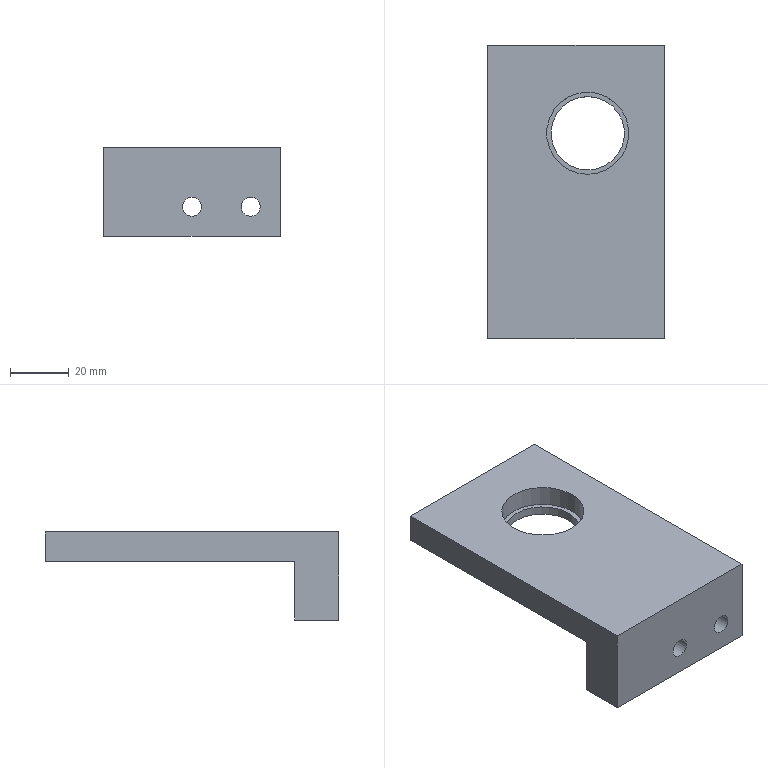Part | NX | features DATUM_CSYS 4, HOLE PACKAGE 3, SKETCH 3, CBORE_HOLE 2, SIMPLE HOLE 2, EXTRUDE 1 | 1 solid | 17 faces | box 60 x 100 x 30 mm | volume 70418 mm3 | plane 11 | cylinder 6 | commonest cylinder face diameters 6.5 x2 11 x2 25 x1 28 x1
STEP:
#1=CARTESIAN_POINT('',(0.,0.,13.25));
#2=VERTEX_POINT('',#1);
#3=CARTESIAN_POINT('',(0.,0.,10.));
#4=DIRECTION('',(0.,1.,0.));
#5=DIRECTION('',(0.,0.,1.));
#6=AXIS2_PLACEMENT_3D('',#3,#4,#5);
#7=CIRCLE('',#6,3.25);
#8=EDGE_CURVE('',#2,#2,#7,.T.);
#9=ORIENTED_EDGE('',*,*,#8,.T.);
#10=EDGE_LOOP('',(#9));
#11=FACE_BOUND('',#10,.T.);
#12=CARTESIAN_POINT('',(20.,0.,13.25));
#13=VERTEX_POINT('',#12);
#14=CARTESIAN_POINT('',(20.,0.,10.));
#15=DIRECTION('',(0.,1.,0.));
#16=DIRECTION('',(0.,0.,1.));
#17=AXIS2_PLACEMENT_3D('',#14,#15,#16);
#18=CIRCLE('',#17,3.25);
#19=EDGE_CURVE('',#13,#13,#18,.T.);
#20=ORIENTED_EDGE('',*,*,#19,.T.);
#21=EDGE_LOOP('',(#20));
#22=FACE_BOUND('',#21,.T.);
#23=CARTESIAN_POINT('',(-30.,0.,30.));
#24=VERTEX_POINT('',#23);
#25=CARTESIAN_POINT('',(-30.,0.,0.));
#26=VERTEX_POINT('',#25);
#27=CARTESIAN_POINT('',(-30.,0.,30.));
#28=DIRECTION('',(0.,0.,-1.));
#29=VECTOR('',#28,1000.);
#30=LINE('',#27,#29);
#31=EDGE_CURVE('',#24,#26,#30,.T.);
#32=ORIENTED_EDGE('',*,*,#31,.T.);
#33=CARTESIAN_POINT('',(30.,0.,0.));
#34=VERTEX_POINT('',#33);
#35=CARTESIAN_POINT('',(30.,0.,0.));
#36=DIRECTION('',(-1.,0.,0.));
#37=VECTOR('',#36,1000.);
#38=LINE('',#35,#37);
#39=EDGE_CURVE('',#34,#26,#38,.T.);
#40=ORIENTED_EDGE('',*,*,#39,.F.);
#41=CARTESIAN_POINT('',(30.,0.,30.));
#42=VERTEX_POINT('',#41);
#43=CARTESIAN_POINT('',(30.,0.,30.));
#44=DIRECTION('',(0.,0.,-1.));
#45=VECTOR('',#44,1000.);
#46=LINE('',#43,#45);
#47=EDGE_CURVE('',#42,#34,#46,.T.);
#48=ORIENTED_EDGE('',*,*,#47,.F.);
#49=CARTESIAN_POINT('',(30.,0.,30.));
#50=DIRECTION('',(-1.,0.,0.));
#51=VECTOR('',#50,1000.);
#52=LINE('',#49,#51);
#53=EDGE_CURVE('',#42,#24,#52,.T.);
#54=ORIENTED_EDGE('',*,*,#53,.T.);
#55=EDGE_LOOP('',(#32,#40,#48,#54));
#56=FACE_BOUND('',#55,.T.);
#57=CARTESIAN_POINT('',(30.,0.,30.));
#58=DIRECTION('',(0.,1.,0.));
#59=DIRECTION('',(0.,0.,1.));
#60=AXIS2_PLACEMENT_3D('',#57,#58,#59);
#61=PLANE('',#60);
#62=ADVANCED_FACE('',(#11,#22,#56),#61,.F.);
#63=CARTESIAN_POINT('',(-30.,15.,0.));
#64=VERTEX_POINT('',#63);
#65=CARTESIAN_POINT('',(-30.,0.,0.));
#66=DIRECTION('',(0.,1.,0.));
#67=VECTOR('',#66,1000.);
#68=LINE('',#65,#67);
#69=EDGE_CURVE('',#26,#64,#68,.T.);
#70=ORIENTED_EDGE('',*,*,#69,.T.);
#71=CARTESIAN_POINT('',(30.,15.,0.));
#72=VERTEX_POINT('',#71);
#73=CARTESIAN_POINT('',(30.,15.,0.));
#74=DIRECTION('',(-1.,0.,0.));
#75=VECTOR('',#74,1000.);
#76=LINE('',#73,#75);
#77=EDGE_CURVE('',#72,#64,#76,.T.);
#78=ORIENTED_EDGE('',*,*,#77,.F.);
#79=CARTESIAN_POINT('',(30.,0.,0.));
#80=DIRECTION('',(0.,1.,0.));
#81=VECTOR('',#80,1000.);
#82=LINE('',#79,#81);
#83=EDGE_CURVE('',#34,#72,#82,.T.);
#84=ORIENTED_EDGE('',*,*,#83,.F.);
#85=ORIENTED_EDGE('',*,*,#39,.T.);
#86=EDGE_LOOP('',(#70,#78,#84,#85));
#87=FACE_BOUND('',#86,.T.);
#88=CARTESIAN_POINT('',(30.,0.,0.));
#89=DIRECTION('',(0.,0.,1.));
#90=DIRECTION('',(0.,-1.,0.));
#91=AXIS2_PLACEMENT_3D('',#88,#89,#90);
#92=PLANE('',#91);
#93=ADVANCED_FACE('',(#87),#92,.F.);
#94=CARTESIAN_POINT('',(0.,15.,4.5));
#95=VERTEX_POINT('',#94);
#96=CARTESIAN_POINT('',(0.,15.,10.));
#97=DIRECTION('',(0.,-1.,0.));
#98=DIRECTION('',(0.,0.,-1.));
#99=AXIS2_PLACEMENT_3D('',#96,#97,#98);
#100=CIRCLE('',#99,5.5);
#101=EDGE_CURVE('',#95,#95,#100,.T.);
#102=ORIENTED_EDGE('',*,*,#101,.T.);
#103=EDGE_LOOP('',(#102));
#104=FACE_BOUND('',#103,.T.);
#105=CARTESIAN_POINT('',(20.,15.,4.5));
#106=VERTEX_POINT('',#105);
#107=CARTESIAN_POINT('',(20.,15.,10.));
#108=DIRECTION('',(0.,-1.,0.));
#109=DIRECTION('',(0.,0.,-1.));
#110=AXIS2_PLACEMENT_3D('',#107,#108,#109);
#111=CIRCLE('',#110,5.5);
#112=EDGE_CURVE('',#106,#106,#111,.T.);
#113=ORIENTED_EDGE('',*,*,#112,.T.);
#114=EDGE_LOOP('',(#113));
#115=FACE_BOUND('',#114,.T.);
#116=CARTESIAN_POINT('',(-30.,15.,20.));
#117=VERTEX_POINT('',#116);
#118=CARTESIAN_POINT('',(-30.,15.,0.));
#119=DIRECTION('',(0.,0.,1.));
#120=VECTOR('',#119,1000.);
#121=LINE('',#118,#120);
#122=EDGE_CURVE('',#64,#117,#121,.T.);
#123=ORIENTED_EDGE('',*,*,#122,.T.);
#124=CARTESIAN_POINT('',(30.,15.,20.));
#125=VERTEX_POINT('',#124);
#126=CARTESIAN_POINT('',(30.,15.,20.));
#127=DIRECTION('',(-1.,0.,0.));
#128=VECTOR('',#127,1000.);
#129=LINE('',#126,#128);
#130=EDGE_CURVE('',#125,#117,#129,.T.);
#131=ORIENTED_EDGE('',*,*,#130,.F.);
#132=CARTESIAN_POINT('',(30.,15.,0.));
#133=DIRECTION('',(0.,0.,1.));
#134=VECTOR('',#133,1000.);
#135=LINE('',#132,#134);
#136=EDGE_CURVE('',#72,#125,#135,.T.);
#137=ORIENTED_EDGE('',*,*,#136,.F.);
#138=ORIENTED_EDGE('',*,*,#77,.T.);
#139=EDGE_LOOP('',(#123,#131,#137,#138));
#140=FACE_BOUND('',#139,.T.);
#141=CARTESIAN_POINT('',(30.,15.,0.));
#142=DIRECTION('',(0.,-1.,0.));
#143=DIRECTION('',(0.,0.,-1.));
#144=AXIS2_PLACEMENT_3D('',#141,#142,#143);
#145=PLANE('',#144);
#146=ADVANCED_FACE('',(#104,#115,#140),#145,.F.);
#147=CARTESIAN_POINT('',(4.,57.5,20.));
#148=VERTEX_POINT('',#147);
#149=CARTESIAN_POINT('',(4.,70.,20.));
#150=DIRECTION('',(0.,0.,1.));
#151=DIRECTION('',(0.,-1.,0.));
#152=AXIS2_PLACEMENT_3D('',#149,#150,#151);
#153=CIRCLE('',#152,12.5);
#154=EDGE_CURVE('',#148,#148,#153,.T.);
#155=ORIENTED_EDGE('',*,*,#154,.T.);
#156=EDGE_LOOP('',(#155));
#157=FACE_BOUND('',#156,.T.);
#158=CARTESIAN_POINT('',(-30.,100.,20.));
#159=VERTEX_POINT('',#158);
#160=CARTESIAN_POINT('',(-30.,15.,20.));
#161=DIRECTION('',(0.,1.,0.));
#162=VECTOR('',#161,1000.);
#163=LINE('',#160,#162);
#164=EDGE_CURVE('',#117,#159,#163,.T.);
#165=ORIENTED_EDGE('',*,*,#164,.T.);
#166=CARTESIAN_POINT('',(30.,100.,20.));
#167=VERTEX_POINT('',#166);
#168=CARTESIAN_POINT('',(30.,100.,20.));
#169=DIRECTION('',(-1.,0.,0.));
#170=VECTOR('',#169,1000.);
#171=LINE('',#168,#170);
#172=EDGE_CURVE('',#167,#159,#171,.T.);
#173=ORIENTED_EDGE('',*,*,#172,.F.);
#174=CARTESIAN_POINT('',(30.,15.,20.));
#175=DIRECTION('',(0.,1.,0.));
#176=VECTOR('',#175,1000.);
#177=LINE('',#174,#176);
#178=EDGE_CURVE('',#125,#167,#177,.T.);
#179=ORIENTED_EDGE('',*,*,#178,.F.);
#180=ORIENTED_EDGE('',*,*,#130,.T.);
#181=EDGE_LOOP('',(#165,#173,#179,#180));
#182=FACE_BOUND('',#181,.T.);
#183=CARTESIAN_POINT('',(30.,15.,20.));
#184=DIRECTION('',(0.,0.,1.));
#185=DIRECTION('',(0.,-1.,0.));
#186=AXIS2_PLACEMENT_3D('',#183,#184,#185);
#187=PLANE('',#186);
#188=ADVANCED_FACE('',(#157,#182),#187,.F.);
#189=CARTESIAN_POINT('',(-30.,100.,30.));
#190=VERTEX_POINT('',#189);
#191=CARTESIAN_POINT('',(-30.,100.,20.));
#192=DIRECTION('',(0.,0.,1.));
#193=VECTOR('',#192,1000.);
#194=LINE('',#191,#193);
#195=EDGE_CURVE('',#159,#190,#194,.T.);
#196=ORIENTED_EDGE('',*,*,#195,.T.);
#197=CARTESIAN_POINT('',(30.,100.,30.));
#198=VERTEX_POINT('',#197);
#199=CARTESIAN_POINT('',(30.,100.,30.));
#200=DIRECTION('',(-1.,0.,0.));
#201=VECTOR('',#200,1000.);
#202=LINE('',#199,#201);
#203=EDGE_CURVE('',#198,#190,#202,.T.);
#204=ORIENTED_EDGE('',*,*,#203,.F.);
#205=CARTESIAN_POINT('',(30.,100.,20.));
#206=DIRECTION('',(0.,0.,1.));
#207=VECTOR('',#206,1000.);
#208=LINE('',#205,#207);
#209=EDGE_CURVE('',#167,#198,#208,.T.);
#210=ORIENTED_EDGE('',*,*,#209,.F.);
#211=ORIENTED_EDGE('',*,*,#172,.T.);
#212=EDGE_LOOP('',(#196,#204,#210,#211));
#213=FACE_BOUND('',#212,.T.);
#214=CARTESIAN_POINT('',(30.,100.,20.));
#215=DIRECTION('',(0.,-1.,0.));
#216=DIRECTION('',(0.,0.,-1.));
#217=AXIS2_PLACEMENT_3D('',#214,#215,#216);
#218=PLANE('',#217);
#219=ADVANCED_FACE('',(#213),#218,.F.);
#220=CARTESIAN_POINT('',(4.,84.,30.));
#221=VERTEX_POINT('',#220);
#222=CARTESIAN_POINT('',(4.,70.,30.));
#223=DIRECTION('',(0.,0.,-1.));
#224=DIRECTION('',(0.,1.,0.));
#225=AXIS2_PLACEMENT_3D('',#222,#223,#224);
#226=CIRCLE('',#225,14.);
#227=EDGE_CURVE('',#221,#221,#226,.T.);
#228=ORIENTED_EDGE('',*,*,#227,.T.);
#229=EDGE_LOOP('',(#228));
#230=FACE_BOUND('',#229,.T.);
#231=CARTESIAN_POINT('',(-30.,100.,30.));
#232=DIRECTION('',(0.,-1.,0.));
#233=VECTOR('',#232,1000.);
#234=LINE('',#231,#233);
#235=EDGE_CURVE('',#190,#24,#234,.T.);
#236=ORIENTED_EDGE('',*,*,#235,.T.);
#237=ORIENTED_EDGE('',*,*,#53,.F.);
#238=CARTESIAN_POINT('',(30.,100.,30.));
#239=DIRECTION('',(0.,-1.,0.));
#240=VECTOR('',#239,1000.);
#241=LINE('',#238,#240);
#242=EDGE_CURVE('',#198,#42,#241,.T.);
#243=ORIENTED_EDGE('',*,*,#242,.F.);
#244=ORIENTED_EDGE('',*,*,#203,.T.);
#245=EDGE_LOOP('',(#236,#237,#243,#244));
#246=FACE_BOUND('',#245,.T.);
#247=CARTESIAN_POINT('',(30.,100.,30.));
#248=DIRECTION('',(0.,0.,-1.));
#249=DIRECTION('',(0.,1.,0.));
#250=AXIS2_PLACEMENT_3D('',#247,#248,#249);
#251=PLANE('',#250);
#252=ADVANCED_FACE('',(#230,#246),#251,.F.);
#253=ORIENTED_EDGE('',*,*,#47,.T.);
#254=ORIENTED_EDGE('',*,*,#83,.T.);
#255=ORIENTED_EDGE('',*,*,#136,.T.);
#256=ORIENTED_EDGE('',*,*,#178,.T.);
#257=ORIENTED_EDGE('',*,*,#209,.T.);
#258=ORIENTED_EDGE('',*,*,#242,.T.);
#259=EDGE_LOOP('',(#253,#254,#255,#256,#257,#258));
#260=FACE_BOUND('',#259,.T.);
#261=CARTESIAN_POINT('',(30.,0.,0.));
#262=DIRECTION('',(1.,0.,0.));
#263=DIRECTION('',(0.,0.,-1.));
#264=AXIS2_PLACEMENT_3D('',#261,#262,#263);
#265=PLANE('',#264);
#266=ADVANCED_FACE('',(#260),#265,.T.);
#267=ORIENTED_EDGE('',*,*,#31,.F.);
#268=ORIENTED_EDGE('',*,*,#235,.F.);
#269=ORIENTED_EDGE('',*,*,#195,.F.);
#270=ORIENTED_EDGE('',*,*,#164,.F.);
#271=ORIENTED_EDGE('',*,*,#122,.F.);
#272=ORIENTED_EDGE('',*,*,#69,.F.);
#273=EDGE_LOOP('',(#267,#268,#269,#270,#271,#272));
#274=FACE_BOUND('',#273,.T.);
#275=CARTESIAN_POINT('',(-30.,0.,0.));
#276=DIRECTION('',(1.,0.,0.));
#277=DIRECTION('',(0.,0.,-1.));
#278=AXIS2_PLACEMENT_3D('',#275,#276,#277);
#279=PLANE('',#278);
#280=ADVANCED_FACE('',(#274),#279,.F.);
#281=CARTESIAN_POINT('',(4.,82.5,23.));
#282=VERTEX_POINT('',#281);
#283=CARTESIAN_POINT('',(4.,70.,23.));
#284=DIRECTION('',(0.,0.,-1.));
#285=DIRECTION('',(0.,1.,0.));
#286=AXIS2_PLACEMENT_3D('',#283,#284,#285);
#287=CIRCLE('',#286,12.5);
#288=EDGE_CURVE('',#282,#282,#287,.T.);
#289=ORIENTED_EDGE('',*,*,#288,.T.);
#290=EDGE_LOOP('',(#289));
#291=FACE_BOUND('',#290,.T.);
#292=CARTESIAN_POINT('',(4.,84.,23.));
#293=VERTEX_POINT('',#292);
#294=CARTESIAN_POINT('',(4.,70.,23.));
#295=DIRECTION('',(0.,0.,-1.));
#296=DIRECTION('',(0.,1.,0.));
#297=AXIS2_PLACEMENT_3D('',#294,#295,#296);
#298=CIRCLE('',#297,14.);
#299=EDGE_CURVE('',#293,#293,#298,.F.);
#300=ORIENTED_EDGE('',*,*,#299,.T.);
#301=EDGE_LOOP('',(#300));
#302=FACE_BOUND('',#301,.T.);
#303=CARTESIAN_POINT('',(4.,70.,23.));
#304=DIRECTION('',(0.,0.,-1.));
#305=DIRECTION('',(0.,1.,0.));
#306=AXIS2_PLACEMENT_3D('',#303,#304,#305);
#307=PLANE('',#306);
#308=ADVANCED_FACE('',(#291,#302),#307,.F.);
#309=ORIENTED_EDGE('',*,*,#299,.F.);
#310=EDGE_LOOP('',(#309));
#311=FACE_BOUND('',#310,.T.);
#312=ORIENTED_EDGE('',*,*,#227,.F.);
#313=EDGE_LOOP('',(#312));
#314=FACE_BOUND('',#313,.T.);
#315=CARTESIAN_POINT('',(4.,70.,30.));
#316=DIRECTION('',(0.,0.,-1.));
#317=DIRECTION('',(0.,1.,0.));
#318=AXIS2_PLACEMENT_3D('',#315,#316,#317);
#319=CYLINDRICAL_SURFACE('',#318,14.);
#320=ADVANCED_FACE('',(#311,#314),#319,.F.);
#321=ORIENTED_EDGE('',*,*,#288,.F.);
#322=EDGE_LOOP('',(#321));
#323=FACE_BOUND('',#322,.T.);
#324=ORIENTED_EDGE('',*,*,#154,.F.);
#325=EDGE_LOOP('',(#324));
#326=FACE_BOUND('',#325,.T.);
#327=CARTESIAN_POINT('',(4.,70.,23.));
#328=DIRECTION('',(0.,0.,-1.));
#329=DIRECTION('',(0.,1.,0.));
#330=AXIS2_PLACEMENT_3D('',#327,#328,#329);
#331=CYLINDRICAL_SURFACE('',#330,12.5);
#332=ADVANCED_FACE('',(#323,#326),#331,.F.);
#333=CARTESIAN_POINT('',(20.,8.5,6.75));
#334=VERTEX_POINT('',#333);
#335=CARTESIAN_POINT('',(20.,8.5,10.));
#336=DIRECTION('',(0.,-1.,0.));
#337=DIRECTION('',(0.,0.,-1.));
#338=AXIS2_PLACEMENT_3D('',#335,#336,#337);
#339=CIRCLE('',#338,3.25);
#340=EDGE_CURVE('',#334,#334,#339,.F.);
#341=ORIENTED_EDGE('',*,*,#340,.T.);
#342=EDGE_LOOP('',(#341));
#343=FACE_BOUND('',#342,.T.);
#344=ORIENTED_EDGE('',*,*,#19,.F.);
#345=EDGE_LOOP('',(#344));
#346=FACE_BOUND('',#345,.T.);
#347=CARTESIAN_POINT('',(20.,-12.938,10.));
#348=DIRECTION('',(0.,-1.,0.));
#349=DIRECTION('',(0.,0.,-1.));
#350=AXIS2_PLACEMENT_3D('',#347,#348,#349);
#351=CYLINDRICAL_SURFACE('',#350,3.25);
#352=ADVANCED_FACE('',(#343,#346),#351,.F.);
#353=ORIENTED_EDGE('',*,*,#340,.F.);
#354=EDGE_LOOP('',(#353));
#355=FACE_BOUND('',#354,.T.);
#356=CARTESIAN_POINT('',(20.,8.5,4.5));
#357=VERTEX_POINT('',#356);
#358=CARTESIAN_POINT('',(20.,8.5,10.));
#359=DIRECTION('',(0.,-1.,0.));
#360=DIRECTION('',(0.,0.,-1.));
#361=AXIS2_PLACEMENT_3D('',#358,#359,#360);
#362=CIRCLE('',#361,5.5);
#363=EDGE_CURVE('',#357,#357,#362,.F.);
#364=ORIENTED_EDGE('',*,*,#363,.T.);
#365=EDGE_LOOP('',(#364));
#366=FACE_BOUND('',#365,.T.);
#367=CARTESIAN_POINT('',(20.,8.5,10.));
#368=DIRECTION('',(0.,-1.,0.));
#369=DIRECTION('',(0.,0.,-1.));
#370=AXIS2_PLACEMENT_3D('',#367,#368,#369);
#371=PLANE('',#370);
#372=ADVANCED_FACE('',(#355,#366),#371,.F.);
#373=ORIENTED_EDGE('',*,*,#363,.F.);
#374=EDGE_LOOP('',(#373));
#375=FACE_BOUND('',#374,.T.);
#376=ORIENTED_EDGE('',*,*,#112,.F.);
#377=EDGE_LOOP('',(#376));
#378=FACE_BOUND('',#377,.T.);
#379=CARTESIAN_POINT('',(20.,15.,10.));
#380=DIRECTION('',(0.,-1.,0.));
#381=DIRECTION('',(0.,0.,-1.));
#382=AXIS2_PLACEMENT_3D('',#379,#380,#381);
#383=CYLINDRICAL_SURFACE('',#382,5.5);
#384=ADVANCED_FACE('',(#375,#378),#383,.F.);
#385=CARTESIAN_POINT('',(0.,8.5,6.75));
#386=VERTEX_POINT('',#385);
#387=CARTESIAN_POINT('',(0.,8.5,10.));
#388=DIRECTION('',(0.,-1.,0.));
#389=DIRECTION('',(0.,0.,-1.));
#390=AXIS2_PLACEMENT_3D('',#387,#388,#389);
#391=CIRCLE('',#390,3.25);
#392=EDGE_CURVE('',#386,#386,#391,.F.);
#393=ORIENTED_EDGE('',*,*,#392,.T.);
#394=EDGE_LOOP('',(#393));
#395=FACE_BOUND('',#394,.T.);
#396=ORIENTED_EDGE('',*,*,#8,.F.);
#397=EDGE_LOOP('',(#396));
#398=FACE_BOUND('',#397,.T.);
#399=CARTESIAN_POINT('',(0.,-16.04,10.));
#400=DIRECTION('',(0.,-1.,0.));
#401=DIRECTION('',(0.,0.,-1.));
#402=AXIS2_PLACEMENT_3D('',#399,#400,#401);
#403=CYLINDRICAL_SURFACE('',#402,3.25);
#404=ADVANCED_FACE('',(#395,#398),#403,.F.);
#405=ORIENTED_EDGE('',*,*,#392,.F.);
#406=EDGE_LOOP('',(#405));
#407=FACE_BOUND('',#406,.T.);
#408=CARTESIAN_POINT('',(0.,8.5,4.5));
#409=VERTEX_POINT('',#408);
#410=CARTESIAN_POINT('',(0.,8.5,10.));
#411=DIRECTION('',(0.,-1.,0.));
#412=DIRECTION('',(0.,0.,-1.));
#413=AXIS2_PLACEMENT_3D('',#410,#411,#412);
#414=CIRCLE('',#413,5.5);
#415=EDGE_CURVE('',#409,#409,#414,.F.);
#416=ORIENTED_EDGE('',*,*,#415,.T.);
#417=EDGE_LOOP('',(#416));
#418=FACE_BOUND('',#417,.T.);
#419=CARTESIAN_POINT('',(0.,8.5,10.));
#420=DIRECTION('',(0.,-1.,0.));
#421=DIRECTION('',(0.,0.,-1.));
#422=AXIS2_PLACEMENT_3D('',#419,#420,#421);
#423=PLANE('',#422);
#424=ADVANCED_FACE('',(#407,#418),#423,.F.);
#425=ORIENTED_EDGE('',*,*,#415,.F.);
#426=EDGE_LOOP('',(#425));
#427=FACE_BOUND('',#426,.T.);
#428=ORIENTED_EDGE('',*,*,#101,.F.);
#429=EDGE_LOOP('',(#428));
#430=FACE_BOUND('',#429,.T.);
#431=CARTESIAN_POINT('',(0.,15.,10.));
#432=DIRECTION('',(0.,-1.,0.));
#433=DIRECTION('',(0.,0.,-1.));
#434=AXIS2_PLACEMENT_3D('',#431,#432,#433);
#435=CYLINDRICAL_SURFACE('',#434,5.5);
#436=ADVANCED_FACE('',(#427,#430),#435,.F.);
#437=CLOSED_SHELL('',(#62,#93,#146,#188,#219,#252,#266,#280,#308,#320,#332,#352,#372,#384,#404,#424,#436));
#438=MANIFOLD_SOLID_BREP('',#437);
#439=(LENGTH_UNIT()NAMED_UNIT(*)SI_UNIT(.MILLI.,.METRE.));
#440=UNCERTAINTY_MEASURE_WITH_UNIT(LENGTH_MEASURE(0.00001),#439,'','');
#441=(NAMED_UNIT(*)PLANE_ANGLE_UNIT()SI_UNIT($,.RADIAN.));
#442=(NAMED_UNIT(*)SI_UNIT($,.STERADIAN.)SOLID_ANGLE_UNIT());
#443=(GEOMETRIC_REPRESENTATION_CONTEXT(3)GLOBAL_UNCERTAINTY_ASSIGNED_CONTEXT((#440))GLOBAL_UNIT_ASSIGNED_CONTEXT((#439,#441,#442))REPRESENTATION_CONTEXT('',''));
#444=ADVANCED_BREP_SHAPE_REPRESENTATION('',(#438),#443);